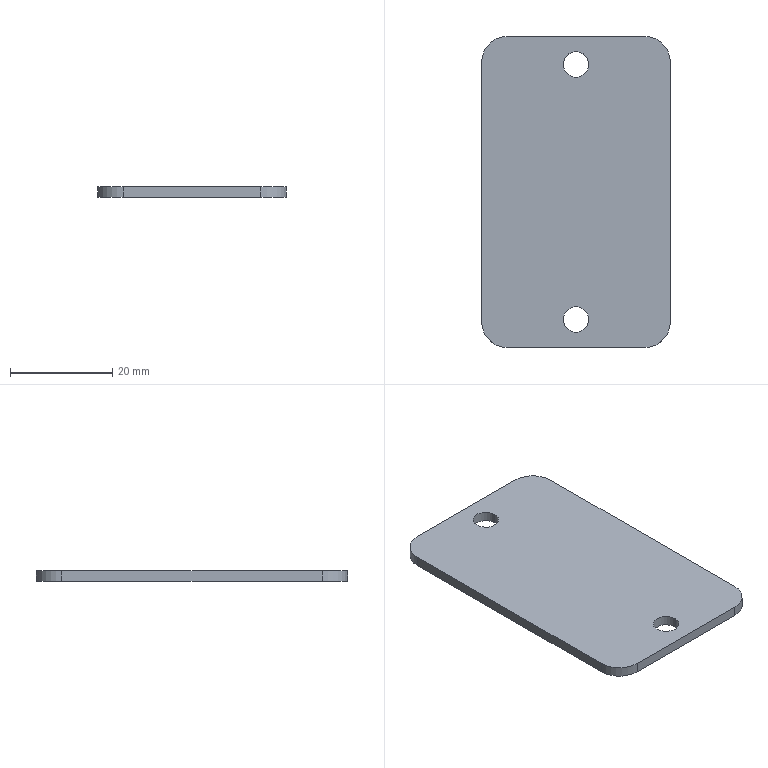Part | NX | features BREP 1 | 1 solid | 14 faces | box 37 x 61 x 2 mm | volume 4393 mm3 | cylinder 8 | plane 6 | commonest cylinder face diameters 5 x4 10 x4
STEP:
#1=CARTESIAN_POINT('',(-143.561,131.716,217.438));
#2=VERTEX_POINT('',#1);
#3=CARTESIAN_POINT('',(-143.561,80.716,217.438));
#4=VERTEX_POINT('',#3);
#5=CARTESIAN_POINT('',(-143.561,106.216,217.438));
#6=DIRECTION('',(0.,-1.,0.));
#7=VECTOR('',#6,1000.);
#8=LINE('',#5,#7);
#9=EDGE_CURVE('',#2,#4,#8,.T.);
#10=ORIENTED_EDGE('',*,*,#9,.T.);
#11=CARTESIAN_POINT('',(-143.561,80.716,219.438));
#12=VERTEX_POINT('',#11);
#13=CARTESIAN_POINT('',(-143.561,80.716,218.438));
#14=DIRECTION('',(0.,0.,-1.));
#15=VECTOR('',#14,1000.);
#16=LINE('',#13,#15);
#17=EDGE_CURVE('',#12,#4,#16,.T.);
#18=ORIENTED_EDGE('',*,*,#17,.F.);
#19=CARTESIAN_POINT('',(-143.561,131.716,219.438));
#20=VERTEX_POINT('',#19);
#21=CARTESIAN_POINT('',(-143.561,106.216,219.438));
#22=DIRECTION('',(0.,-1.,0.));
#23=VECTOR('',#22,1000.);
#24=LINE('',#21,#23);
#25=EDGE_CURVE('',#20,#12,#24,.T.);
#26=ORIENTED_EDGE('',*,*,#25,.F.);
#27=CARTESIAN_POINT('',(-143.561,131.716,218.438));
#28=DIRECTION('',(0.,0.,-1.));
#29=VECTOR('',#28,1000.);
#30=LINE('',#27,#29);
#31=EDGE_CURVE('',#20,#2,#30,.T.);
#32=ORIENTED_EDGE('',*,*,#31,.T.);
#33=EDGE_LOOP('',(#10,#18,#26,#32));
#34=FACE_BOUND('',#33,.T.);
#35=CARTESIAN_POINT('',(-143.561,131.716,219.438));
#36=DIRECTION('',(1.,0.,0.));
#37=DIRECTION('',(0.,1.,0.));
#38=AXIS2_PLACEMENT_3D('',#35,#36,#37);
#39=PLANE('',#38);
#40=ADVANCED_FACE('',(#34),#39,.F.);
#41=ORIENTED_EDGE('',*,*,#9,.F.);
#42=CARTESIAN_POINT('',(-138.561,136.716,217.438));
#43=VERTEX_POINT('',#42);
#44=CARTESIAN_POINT('',(-138.561,131.716,217.438));
#45=DIRECTION('',(0.,0.,1.));
#46=DIRECTION('',(1.,0.,0.));
#47=AXIS2_PLACEMENT_3D('',#44,#45,#46);
#48=CIRCLE('',#47,5.);
#49=EDGE_CURVE('',#43,#2,#48,.T.);
#50=ORIENTED_EDGE('',*,*,#49,.F.);
#51=CARTESIAN_POINT('',(-111.561,136.716,217.438));
#52=VERTEX_POINT('',#51);
#53=CARTESIAN_POINT('',(-125.061,136.716,217.438));
#54=DIRECTION('',(-1.,0.,0.));
#55=VECTOR('',#54,1000.);
#56=LINE('',#53,#55);
#57=EDGE_CURVE('',#52,#43,#56,.T.);
#58=ORIENTED_EDGE('',*,*,#57,.F.);
#59=CARTESIAN_POINT('',(-106.561,131.716,217.438));
#60=VERTEX_POINT('',#59);
#61=CARTESIAN_POINT('',(-111.561,131.716,217.438));
#62=DIRECTION('',(0.,0.,1.));
#63=DIRECTION('',(1.,0.,0.));
#64=AXIS2_PLACEMENT_3D('',#61,#62,#63);
#65=CIRCLE('',#64,5.);
#66=EDGE_CURVE('',#60,#52,#65,.T.);
#67=ORIENTED_EDGE('',*,*,#66,.F.);
#68=CARTESIAN_POINT('',(-106.561,80.716,217.438));
#69=VERTEX_POINT('',#68);
#70=CARTESIAN_POINT('',(-106.561,106.216,217.438));
#71=DIRECTION('',(0.,1.,0.));
#72=VECTOR('',#71,1000.);
#73=LINE('',#70,#72);
#74=EDGE_CURVE('',#69,#60,#73,.T.);
#75=ORIENTED_EDGE('',*,*,#74,.F.);
#76=CARTESIAN_POINT('',(-111.561,75.716,217.438));
#77=VERTEX_POINT('',#76);
#78=CARTESIAN_POINT('',(-111.561,80.716,217.438));
#79=DIRECTION('',(0.,0.,1.));
#80=DIRECTION('',(1.,0.,0.));
#81=AXIS2_PLACEMENT_3D('',#78,#79,#80);
#82=CIRCLE('',#81,5.);
#83=EDGE_CURVE('',#77,#69,#82,.T.);
#84=ORIENTED_EDGE('',*,*,#83,.F.);
#85=CARTESIAN_POINT('',(-138.561,75.716,217.438));
#86=VERTEX_POINT('',#85);
#87=CARTESIAN_POINT('',(-125.061,75.716,217.438));
#88=DIRECTION('',(1.,0.,0.));
#89=VECTOR('',#88,1000.);
#90=LINE('',#87,#89);
#91=EDGE_CURVE('',#86,#77,#90,.T.);
#92=ORIENTED_EDGE('',*,*,#91,.F.);
#93=CARTESIAN_POINT('',(-138.561,80.716,217.438));
#94=DIRECTION('',(0.,0.,1.));
#95=DIRECTION('',(1.,0.,0.));
#96=AXIS2_PLACEMENT_3D('',#93,#94,#95);
#97=CIRCLE('',#96,5.);
#98=EDGE_CURVE('',#4,#86,#97,.T.);
#99=ORIENTED_EDGE('',*,*,#98,.F.);
#100=EDGE_LOOP('',(#41,#50,#58,#67,#75,#84,#92,#99));
#101=FACE_BOUND('',#100,.T.);
#102=CARTESIAN_POINT('',(-122.561,131.216,217.438));
#103=VERTEX_POINT('',#102);
#104=CARTESIAN_POINT('',(-127.561,131.216,217.438));
#105=VERTEX_POINT('',#104);
#106=CARTESIAN_POINT('',(-125.061,131.216,217.438));
#107=DIRECTION('',(0.,0.,1.));
#108=DIRECTION('',(1.,0.,0.));
#109=AXIS2_PLACEMENT_3D('',#106,#107,#108);
#110=CIRCLE('',#109,2.5);
#111=EDGE_CURVE('',#103,#105,#110,.T.);
#112=ORIENTED_EDGE('',*,*,#111,.T.);
#113=CARTESIAN_POINT('',(-125.061,131.216,217.438));
#114=DIRECTION('',(0.,0.,1.));
#115=DIRECTION('',(1.,0.,0.));
#116=AXIS2_PLACEMENT_3D('',#113,#114,#115);
#117=CIRCLE('',#116,2.5);
#118=EDGE_CURVE('',#105,#103,#117,.T.);
#119=ORIENTED_EDGE('',*,*,#118,.T.);
#120=EDGE_LOOP('',(#112,#119));
#121=FACE_BOUND('',#120,.T.);
#122=CARTESIAN_POINT('',(-122.561,81.216,217.438));
#123=VERTEX_POINT('',#122);
#124=CARTESIAN_POINT('',(-127.561,81.216,217.438));
#125=VERTEX_POINT('',#124);
#126=CARTESIAN_POINT('',(-125.061,81.216,217.438));
#127=DIRECTION('',(0.,0.,1.));
#128=DIRECTION('',(1.,0.,0.));
#129=AXIS2_PLACEMENT_3D('',#126,#127,#128);
#130=CIRCLE('',#129,2.5);
#131=EDGE_CURVE('',#123,#125,#130,.T.);
#132=ORIENTED_EDGE('',*,*,#131,.T.);
#133=CARTESIAN_POINT('',(-125.061,81.216,217.438));
#134=DIRECTION('',(0.,0.,1.));
#135=DIRECTION('',(1.,0.,0.));
#136=AXIS2_PLACEMENT_3D('',#133,#134,#135);
#137=CIRCLE('',#136,2.5);
#138=EDGE_CURVE('',#125,#123,#137,.T.);
#139=ORIENTED_EDGE('',*,*,#138,.T.);
#140=EDGE_LOOP('',(#132,#139));
#141=FACE_BOUND('',#140,.T.);
#142=CARTESIAN_POINT('',(-138.561,80.716,217.438));
#143=DIRECTION('',(0.,0.,1.));
#144=DIRECTION('',(1.,0.,0.));
#145=AXIS2_PLACEMENT_3D('',#142,#143,#144);
#146=PLANE('',#145);
#147=ADVANCED_FACE('',(#101,#121,#141),#146,.F.);
#148=ORIENTED_EDGE('',*,*,#98,.T.);
#149=CARTESIAN_POINT('',(-138.561,75.716,219.438));
#150=VERTEX_POINT('',#149);
#151=CARTESIAN_POINT('',(-138.561,75.716,219.438));
#152=DIRECTION('',(0.,0.,-1.));
#153=VECTOR('',#152,1000.);
#154=LINE('',#151,#153);
#155=EDGE_CURVE('',#150,#86,#154,.T.);
#156=ORIENTED_EDGE('',*,*,#155,.F.);
#157=CARTESIAN_POINT('',(-138.561,80.716,219.438));
#158=DIRECTION('',(0.,0.,1.));
#159=DIRECTION('',(-1.,0.,0.));
#160=AXIS2_PLACEMENT_3D('',#157,#158,#159);
#161=CIRCLE('',#160,5.);
#162=EDGE_CURVE('',#12,#150,#161,.T.);
#163=ORIENTED_EDGE('',*,*,#162,.F.);
#164=ORIENTED_EDGE('',*,*,#17,.T.);
#165=EDGE_LOOP('',(#148,#156,#163,#164));
#166=FACE_BOUND('',#165,.T.);
#167=CARTESIAN_POINT('',(-138.561,80.716,219.438));
#168=DIRECTION('',(0.,0.,-1.));
#169=DIRECTION('',(1.,0.,0.));
#170=AXIS2_PLACEMENT_3D('',#167,#168,#169);
#171=CYLINDRICAL_SURFACE('',#170,5.);
#172=ADVANCED_FACE('',(#166),#171,.T.);
#173=ORIENTED_EDGE('',*,*,#25,.T.);
#174=ORIENTED_EDGE('',*,*,#162,.T.);
#175=CARTESIAN_POINT('',(-111.561,75.716,219.438));
#176=VERTEX_POINT('',#175);
#177=CARTESIAN_POINT('',(-125.061,75.716,219.438));
#178=DIRECTION('',(1.,0.,0.));
#179=VECTOR('',#178,1000.);
#180=LINE('',#177,#179);
#181=EDGE_CURVE('',#150,#176,#180,.T.);
#182=ORIENTED_EDGE('',*,*,#181,.T.);
#183=CARTESIAN_POINT('',(-106.561,80.716,219.438));
#184=VERTEX_POINT('',#183);
#185=CARTESIAN_POINT('',(-111.561,80.716,219.438));
#186=DIRECTION('',(0.,0.,1.));
#187=DIRECTION('',(1.,0.,0.));
#188=AXIS2_PLACEMENT_3D('',#185,#186,#187);
#189=CIRCLE('',#188,5.);
#190=EDGE_CURVE('',#176,#184,#189,.T.);
#191=ORIENTED_EDGE('',*,*,#190,.T.);
#192=CARTESIAN_POINT('',(-106.561,131.716,219.438));
#193=VERTEX_POINT('',#192);
#194=CARTESIAN_POINT('',(-106.561,106.216,219.438));
#195=DIRECTION('',(0.,1.,0.));
#196=VECTOR('',#195,1000.);
#197=LINE('',#194,#196);
#198=EDGE_CURVE('',#184,#193,#197,.T.);
#199=ORIENTED_EDGE('',*,*,#198,.T.);
#200=CARTESIAN_POINT('',(-111.561,136.716,219.438));
#201=VERTEX_POINT('',#200);
#202=CARTESIAN_POINT('',(-111.561,131.716,219.438));
#203=DIRECTION('',(0.,0.,1.));
#204=DIRECTION('',(1.,0.,0.));
#205=AXIS2_PLACEMENT_3D('',#202,#203,#204);
#206=CIRCLE('',#205,5.);
#207=EDGE_CURVE('',#193,#201,#206,.T.);
#208=ORIENTED_EDGE('',*,*,#207,.T.);
#209=CARTESIAN_POINT('',(-138.561,136.716,219.438));
#210=VERTEX_POINT('',#209);
#211=CARTESIAN_POINT('',(-125.061,136.716,219.438));
#212=DIRECTION('',(-1.,0.,0.));
#213=VECTOR('',#212,1000.);
#214=LINE('',#211,#213);
#215=EDGE_CURVE('',#201,#210,#214,.T.);
#216=ORIENTED_EDGE('',*,*,#215,.T.);
#217=CARTESIAN_POINT('',(-138.561,131.716,219.438));
#218=DIRECTION('',(0.,0.,1.));
#219=DIRECTION('',(1.,0.,0.));
#220=AXIS2_PLACEMENT_3D('',#217,#218,#219);
#221=CIRCLE('',#220,5.);
#222=EDGE_CURVE('',#210,#20,#221,.T.);
#223=ORIENTED_EDGE('',*,*,#222,.T.);
#224=EDGE_LOOP('',(#173,#174,#182,#191,#199,#208,#216,#223));
#225=FACE_BOUND('',#224,.T.);
#226=CARTESIAN_POINT('',(-127.561,131.216,219.438));
#227=VERTEX_POINT('',#226);
#228=CARTESIAN_POINT('',(-122.561,131.216,219.438));
#229=VERTEX_POINT('',#228);
#230=CARTESIAN_POINT('',(-125.061,131.216,219.438));
#231=DIRECTION('',(0.,0.,1.));
#232=DIRECTION('',(1.,0.,0.));
#233=AXIS2_PLACEMENT_3D('',#230,#231,#232);
#234=CIRCLE('',#233,2.5);
#235=EDGE_CURVE('',#227,#229,#234,.T.);
#236=ORIENTED_EDGE('',*,*,#235,.F.);
#237=CARTESIAN_POINT('',(-125.061,131.216,219.438));
#238=DIRECTION('',(0.,0.,1.));
#239=DIRECTION('',(1.,0.,0.));
#240=AXIS2_PLACEMENT_3D('',#237,#238,#239);
#241=CIRCLE('',#240,2.5);
#242=EDGE_CURVE('',#229,#227,#241,.T.);
#243=ORIENTED_EDGE('',*,*,#242,.F.);
#244=EDGE_LOOP('',(#236,#243));
#245=FACE_BOUND('',#244,.T.);
#246=CARTESIAN_POINT('',(-127.561,81.216,219.438));
#247=VERTEX_POINT('',#246);
#248=CARTESIAN_POINT('',(-122.561,81.216,219.438));
#249=VERTEX_POINT('',#248);
#250=CARTESIAN_POINT('',(-125.061,81.216,219.438));
#251=DIRECTION('',(0.,0.,1.));
#252=DIRECTION('',(1.,0.,0.));
#253=AXIS2_PLACEMENT_3D('',#250,#251,#252);
#254=CIRCLE('',#253,2.5);
#255=EDGE_CURVE('',#247,#249,#254,.T.);
#256=ORIENTED_EDGE('',*,*,#255,.F.);
#257=CARTESIAN_POINT('',(-125.061,81.216,219.438));
#258=DIRECTION('',(0.,0.,1.));
#259=DIRECTION('',(1.,0.,0.));
#260=AXIS2_PLACEMENT_3D('',#257,#258,#259);
#261=CIRCLE('',#260,2.5);
#262=EDGE_CURVE('',#249,#247,#261,.T.);
#263=ORIENTED_EDGE('',*,*,#262,.F.);
#264=EDGE_LOOP('',(#256,#263));
#265=FACE_BOUND('',#264,.T.);
#266=CARTESIAN_POINT('',(-138.561,80.716,219.438));
#267=DIRECTION('',(0.,0.,1.));
#268=DIRECTION('',(1.,0.,0.));
#269=AXIS2_PLACEMENT_3D('',#266,#267,#268);
#270=PLANE('',#269);
#271=ADVANCED_FACE('',(#225,#245,#265),#270,.T.);
#272=ORIENTED_EDGE('',*,*,#49,.T.);
#273=ORIENTED_EDGE('',*,*,#31,.F.);
#274=ORIENTED_EDGE('',*,*,#222,.F.);
#275=CARTESIAN_POINT('',(-138.561,136.716,219.438));
#276=DIRECTION('',(0.,0.,-1.));
#277=VECTOR('',#276,1000.);
#278=LINE('',#275,#277);
#279=EDGE_CURVE('',#210,#43,#278,.T.);
#280=ORIENTED_EDGE('',*,*,#279,.T.);
#281=EDGE_LOOP('',(#272,#273,#274,#280));
#282=FACE_BOUND('',#281,.T.);
#283=CARTESIAN_POINT('',(-138.561,131.716,219.438));
#284=DIRECTION('',(0.,0.,-1.));
#285=DIRECTION('',(-1.,0.,0.));
#286=AXIS2_PLACEMENT_3D('',#283,#284,#285);
#287=CYLINDRICAL_SURFACE('',#286,5.);
#288=ADVANCED_FACE('',(#282),#287,.T.);
#289=ORIENTED_EDGE('',*,*,#57,.T.);
#290=ORIENTED_EDGE('',*,*,#279,.F.);
#291=ORIENTED_EDGE('',*,*,#215,.F.);
#292=CARTESIAN_POINT('',(-111.561,136.716,218.438));
#293=DIRECTION('',(0.,0.,-1.));
#294=VECTOR('',#293,1000.);
#295=LINE('',#292,#294);
#296=EDGE_CURVE('',#201,#52,#295,.T.);
#297=ORIENTED_EDGE('',*,*,#296,.T.);
#298=EDGE_LOOP('',(#289,#290,#291,#297));
#299=FACE_BOUND('',#298,.T.);
#300=CARTESIAN_POINT('',(-111.561,136.716,219.438));
#301=DIRECTION('',(0.,-1.,0.));
#302=DIRECTION('',(0.,0.,-1.));
#303=AXIS2_PLACEMENT_3D('',#300,#301,#302);
#304=PLANE('',#303);
#305=ADVANCED_FACE('',(#299),#304,.F.);
#306=ORIENTED_EDGE('',*,*,#66,.T.);
#307=ORIENTED_EDGE('',*,*,#296,.F.);
#308=ORIENTED_EDGE('',*,*,#207,.F.);
#309=CARTESIAN_POINT('',(-106.561,131.716,219.438));
#310=DIRECTION('',(0.,0.,-1.));
#311=VECTOR('',#310,1000.);
#312=LINE('',#309,#311);
#313=EDGE_CURVE('',#193,#60,#312,.T.);
#314=ORIENTED_EDGE('',*,*,#313,.T.);
#315=EDGE_LOOP('',(#306,#307,#308,#314));
#316=FACE_BOUND('',#315,.T.);
#317=CARTESIAN_POINT('',(-111.561,131.716,219.438));
#318=DIRECTION('',(0.,0.,-1.));
#319=DIRECTION('',(-1.,0.,0.));
#320=AXIS2_PLACEMENT_3D('',#317,#318,#319);
#321=CYLINDRICAL_SURFACE('',#320,5.);
#322=ADVANCED_FACE('',(#316),#321,.T.);
#323=ORIENTED_EDGE('',*,*,#74,.T.);
#324=ORIENTED_EDGE('',*,*,#313,.F.);
#325=ORIENTED_EDGE('',*,*,#198,.F.);
#326=CARTESIAN_POINT('',(-106.561,80.716,218.438));
#327=DIRECTION('',(0.,0.,-1.));
#328=VECTOR('',#327,1000.);
#329=LINE('',#326,#328);
#330=EDGE_CURVE('',#184,#69,#329,.T.);
#331=ORIENTED_EDGE('',*,*,#330,.T.);
#332=EDGE_LOOP('',(#323,#324,#325,#331));
#333=FACE_BOUND('',#332,.T.);
#334=CARTESIAN_POINT('',(-106.561,80.716,219.438));
#335=DIRECTION('',(-1.,0.,0.));
#336=DIRECTION('',(0.,-1.,0.));
#337=AXIS2_PLACEMENT_3D('',#334,#335,#336);
#338=PLANE('',#337);
#339=ADVANCED_FACE('',(#333),#338,.F.);
#340=ORIENTED_EDGE('',*,*,#83,.T.);
#341=ORIENTED_EDGE('',*,*,#330,.F.);
#342=ORIENTED_EDGE('',*,*,#190,.F.);
#343=CARTESIAN_POINT('',(-111.561,75.716,219.438));
#344=DIRECTION('',(0.,0.,-1.));
#345=VECTOR('',#344,1000.);
#346=LINE('',#343,#345);
#347=EDGE_CURVE('',#176,#77,#346,.T.);
#348=ORIENTED_EDGE('',*,*,#347,.T.);
#349=EDGE_LOOP('',(#340,#341,#342,#348));
#350=FACE_BOUND('',#349,.T.);
#351=CARTESIAN_POINT('',(-111.561,80.716,219.438));
#352=DIRECTION('',(0.,0.,-1.));
#353=DIRECTION('',(1.,0.,0.));
#354=AXIS2_PLACEMENT_3D('',#351,#352,#353);
#355=CYLINDRICAL_SURFACE('',#354,5.);
#356=ADVANCED_FACE('',(#350),#355,.T.);
#357=ORIENTED_EDGE('',*,*,#91,.T.);
#358=ORIENTED_EDGE('',*,*,#347,.F.);
#359=ORIENTED_EDGE('',*,*,#181,.F.);
#360=ORIENTED_EDGE('',*,*,#155,.T.);
#361=EDGE_LOOP('',(#357,#358,#359,#360));
#362=FACE_BOUND('',#361,.T.);
#363=CARTESIAN_POINT('',(-138.561,75.716,219.438));
#364=DIRECTION('',(0.,1.,0.));
#365=DIRECTION('',(0.,0.,1.));
#366=AXIS2_PLACEMENT_3D('',#363,#364,#365);
#367=PLANE('',#366);
#368=ADVANCED_FACE('',(#362),#367,.F.);
#369=ORIENTED_EDGE('',*,*,#111,.F.);
#370=CARTESIAN_POINT('',(-122.561,131.216,219.438));
#371=DIRECTION('',(0.,0.,-1.));
#372=VECTOR('',#371,1000.);
#373=LINE('',#370,#372);
#374=EDGE_CURVE('',#229,#103,#373,.T.);
#375=ORIENTED_EDGE('',*,*,#374,.F.);
#376=ORIENTED_EDGE('',*,*,#242,.T.);
#377=CARTESIAN_POINT('',(-127.561,131.216,219.438));
#378=DIRECTION('',(0.,0.,1.));
#379=VECTOR('',#378,1000.);
#380=LINE('',#377,#379);
#381=EDGE_CURVE('',#105,#227,#380,.T.);
#382=ORIENTED_EDGE('',*,*,#381,.F.);
#383=EDGE_LOOP('',(#369,#375,#376,#382));
#384=FACE_BOUND('',#383,.T.);
#385=CARTESIAN_POINT('',(-125.061,131.216,219.438));
#386=DIRECTION('',(0.,0.,-1.));
#387=DIRECTION('',(-1.,0.,0.));
#388=AXIS2_PLACEMENT_3D('',#385,#386,#387);
#389=CYLINDRICAL_SURFACE('',#388,2.5);
#390=ADVANCED_FACE('',(#384),#389,.F.);
#391=ORIENTED_EDGE('',*,*,#118,.F.);
#392=ORIENTED_EDGE('',*,*,#381,.T.);
#393=ORIENTED_EDGE('',*,*,#235,.T.);
#394=ORIENTED_EDGE('',*,*,#374,.T.);
#395=EDGE_LOOP('',(#391,#392,#393,#394));
#396=FACE_BOUND('',#395,.T.);
#397=CARTESIAN_POINT('',(-125.061,131.216,219.438));
#398=DIRECTION('',(0.,0.,-1.));
#399=DIRECTION('',(1.,0.,0.));
#400=AXIS2_PLACEMENT_3D('',#397,#398,#399);
#401=CYLINDRICAL_SURFACE('',#400,2.5);
#402=ADVANCED_FACE('',(#396),#401,.F.);
#403=ORIENTED_EDGE('',*,*,#131,.F.);
#404=CARTESIAN_POINT('',(-122.561,81.216,219.438));
#405=DIRECTION('',(0.,0.,-1.));
#406=VECTOR('',#405,1000.);
#407=LINE('',#404,#406);
#408=EDGE_CURVE('',#249,#123,#407,.T.);
#409=ORIENTED_EDGE('',*,*,#408,.F.);
#410=ORIENTED_EDGE('',*,*,#262,.T.);
#411=CARTESIAN_POINT('',(-127.561,81.216,219.438));
#412=DIRECTION('',(0.,0.,1.));
#413=VECTOR('',#412,1000.);
#414=LINE('',#411,#413);
#415=EDGE_CURVE('',#125,#247,#414,.T.);
#416=ORIENTED_EDGE('',*,*,#415,.F.);
#417=EDGE_LOOP('',(#403,#409,#410,#416));
#418=FACE_BOUND('',#417,.T.);
#419=CARTESIAN_POINT('',(-125.061,81.216,219.438));
#420=DIRECTION('',(0.,0.,-1.));
#421=DIRECTION('',(-1.,0.,0.));
#422=AXIS2_PLACEMENT_3D('',#419,#420,#421);
#423=CYLINDRICAL_SURFACE('',#422,2.5);
#424=ADVANCED_FACE('',(#418),#423,.F.);
#425=ORIENTED_EDGE('',*,*,#138,.F.);
#426=ORIENTED_EDGE('',*,*,#415,.T.);
#427=ORIENTED_EDGE('',*,*,#255,.T.);
#428=ORIENTED_EDGE('',*,*,#408,.T.);
#429=EDGE_LOOP('',(#425,#426,#427,#428));
#430=FACE_BOUND('',#429,.T.);
#431=CARTESIAN_POINT('',(-125.061,81.216,219.438));
#432=DIRECTION('',(0.,0.,-1.));
#433=DIRECTION('',(1.,0.,0.));
#434=AXIS2_PLACEMENT_3D('',#431,#432,#433);
#435=CYLINDRICAL_SURFACE('',#434,2.5);
#436=ADVANCED_FACE('',(#430),#435,.F.);
#437=CLOSED_SHELL('',(#40,#147,#172,#271,#288,#305,#322,#339,#356,#368,#390,#402,#424,#436));
#438=MANIFOLD_SOLID_BREP('',#437);
#439=(LENGTH_UNIT()NAMED_UNIT(*)SI_UNIT(.MILLI.,.METRE.));
#440=UNCERTAINTY_MEASURE_WITH_UNIT(LENGTH_MEASURE(0.00001),#439,'','');
#441=(NAMED_UNIT(*)PLANE_ANGLE_UNIT()SI_UNIT($,.RADIAN.));
#442=(NAMED_UNIT(*)SI_UNIT($,.STERADIAN.)SOLID_ANGLE_UNIT());
#443=(GEOMETRIC_REPRESENTATION_CONTEXT(3)GLOBAL_UNCERTAINTY_ASSIGNED_CONTEXT((#440))GLOBAL_UNIT_ASSIGNED_CONTEXT((#439,#441,#442))REPRESENTATION_CONTEXT('',''));
#444=ADVANCED_BREP_SHAPE_REPRESENTATION('',(#438),#443);